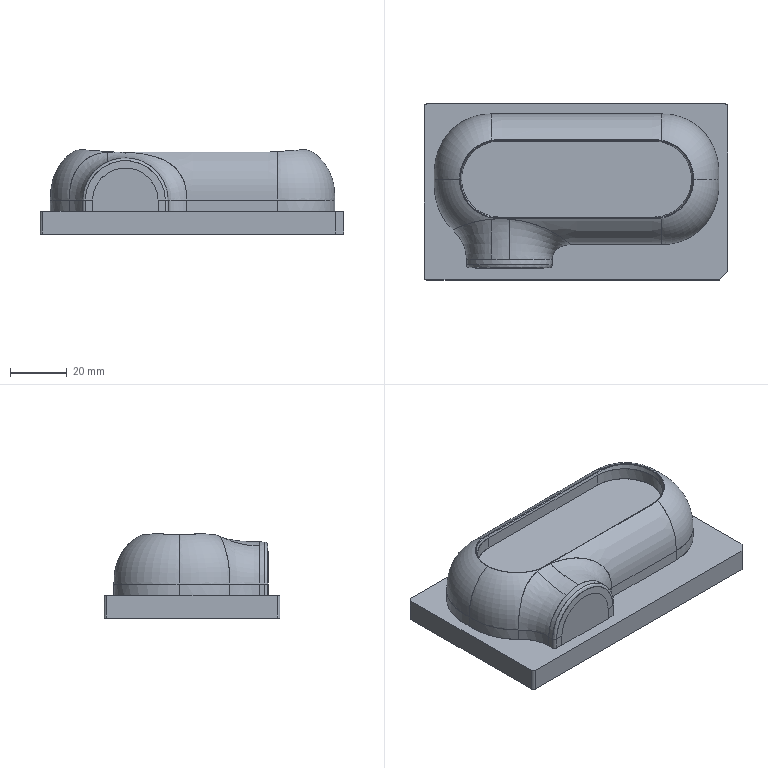NC program | PowerMill | posted by the shop | part box 107 x 62 x 29.663 mm
Lines 34277 to 35410 of 415021:
( TOOL ID   D10_1_1_1 )
( TOOL DIA. 10. TIP RAD 0 LENGTH 84.84 )
( Z = -6.359 )
T3 M6
T17
G91 G28 Z0
G0 G90 G54
M08
S8500 M3
X0 Y0 M8
G43 Z11.802 H3
X-19.327 Y8.267
Z-5.059
G1 Z-6.259 F360
X-25.057 Y8.319 Z-6.359
G3 X-28.917 Y4.509 I-.035 J-3.825 F600
X-25.087 Y.668 I3.825 J-.015
G1 X25.805 Y.724
G3 X25.833 Y7.858 I-.004 J3.567
G1 X-25.057 Y8.319
X-25.019 Y12.498
X-27.025 Y12.494
X-27.593 Y12.467
G3 X-28.444 Y12.348 I.713 J-8.214
G1 X-28.728 Y12.288
G3 X-29.42 Y12.093 I1.854 J-7.911
G1 X-29.863 Y11.932
G3 X-30.431 Y11.681 I3.427 J-8.517
X-30.999 Y11.374 I4.054 J-8.174
G1 X-31.282 Y11.197
X-31.615 Y10.968
X-31.884 Y10.763
X-32.134 Y10.557
X-32.304 Y10.406
X-32.503 Y10.218
X-32.701 Y10.017
X-32.869 Y9.835
X-33.074 Y9.598
X-33.323 Y9.281
X-33.524 Y8.999
X-33.707 Y8.718
X-33.837 Y8.502
X-34.025 Y8.156
X-34.163 Y7.875
X-34.287 Y7.593
X-34.404 Y7.3
X-34.499 Y7.031
X-34.587 Y6.75
X-34.663 Y6.47
X-34.73 Y6.187
G3 X-34.864 Y5.359 I8.12 J-1.736
G1 X-34.905 Y4.781
Y4.219
X-34.866 Y3.656
X-34.831 Y3.375
X-34.785 Y3.093
X-34.73 Y2.813
G3 X-34.404 Y1.7 I8.131 J1.778
G1 X-34.287 Y1.407
G3 X-34.025 Y.844 I8.475 J3.609
G1 X-33.837 Y.498
X-33.707 Y.282
X-33.524 Y.001
X-33.269 Y-.353
G3 X-32.863 Y-.843 I7.187 J5.55
G1 X-32.701 Y-1.017
X-32.503 Y-1.218
G3 X-31.566 Y-2.003 I5.801 J5.972
G1 X-31.282 Y-2.197
G3 X-30.037 Y-2.859 I4.373 J6.723
G1 X-29.863 Y-2.932
X-29.42 Y-3.093
G3 X-28.444 Y-3.348 I2.55 J7.756
G1 X-28.16 Y-3.398
X-27.593 Y-3.467
X-27.309 Y-3.485
X-27.025 Y-3.494
X-26.458 Y-3.498
X27.248 Y-3.496
X27.599 Y-3.49
X27.816 Y-3.482
X28.033 Y-3.467
X28.317 Y-3.438
X28.601 Y-3.398
X28.884 Y-3.348
G3 X29.86 Y-3.093 I-1.564 J7.957
G1 X30.303 Y-2.932
X30.589 Y-2.811
X30.871 Y-2.681
X31.164 Y-2.53
X31.439 Y-2.374
X31.722 Y-2.197
X32.055 Y-1.968
X32.314 Y-1.771
G3 X32.773 Y-1.379 I-5.391 J6.764
G1 X32.943 Y-1.218
X33.148 Y-1.011
X33.304 Y-.843
X33.514 Y-.598
X33.763 Y-.281
X33.964 Y.001
X34.147 Y.282
X34.277 Y.498
X34.465 Y.844
X34.603 Y1.125
X34.728 Y1.407
G3 X34.939 Y1.969 I-8.211 J3.408
G1 X35.026 Y2.249
X35.104 Y2.531
G3 X35.269 Y3.365 I-8.092 J2.037
G1 X35.306 Y3.656
X35.345 Y4.219
Y4.781
X35.306 Y5.344
X35.27 Y5.626
X35.226 Y5.906
G3 X34.947 Y7.007 I-8.097 J-1.467
G1 X34.844 Y7.3
G3 X34.603 Y7.875 I-8.957 J-3.416
G1 X34.465 Y8.156
X34.277 Y8.502
X34.147 Y8.718
X33.964 Y8.999
X33.763 Y9.281
G3 X33.141 Y10.017 I-6.537 J-4.887
G1 X32.943 Y10.218
X32.745 Y10.406
X32.532 Y10.591
X32.314 Y10.771
X32.055 Y10.968
G3 X31.439 Y11.374 I-5.546 J-7.74
G1 X31.164 Y11.53
X30.871 Y11.681
X30.589 Y11.811
X30.303 Y11.932
X30.02 Y12.035
X29.736 Y12.133
G3 X28.884 Y12.348 I-2.437 J-7.865
G1 X28.601 Y12.398
X28.317 Y12.437
X28.033 Y12.467
X27.465 Y12.494
X26.898 Y12.498
X-25.019
X-25.057 Y8.319
G0 Z11.802
X0 Y0
Z9.784
X64.2 Y6.547
Z-20.66
G1 Z-21.86 F360
X58.925 F600
X55.775 Y6.525
X55.776 Y2.383
G2 X55.632 Y-.364 I-30.159 J.203
G1 X55.555 Y-1.057
X55.471 Y-1.684
X55.374 Y-2.309
X55.263 Y-2.93
X55.144 Y-3.525
X55.011 Y-4.118
X54.897 Y-4.589
X54.767 Y-5.079
X54.63 Y-5.568
G2 X53.817 Y-7.944 I-26.15 J7.621
X52.595 Y-10.601 I-24.535 J9.675
G1 X52.226 Y-11.275
X51.836 Y-11.938
X51.516 Y-12.452
X51.249 Y-12.86
X50.861 Y-13.425
X50.457 Y-13.98
X50.035 Y-14.526
X49.535 Y-15.138
X49.502 Y-15.176
X53.081 Y-18.384
G2 X54.12 Y-18.799 I.444 J-.398
G1 X53.881 Y-27.29
G2 X53.366 Y-28.574 I-1.999 J.056
G1 X51.521 Y-30.619
G2 X50.862 Y-31.101 I-1.485 J1.34
G1 X50.317 Y-31.347
G2 X49.495 Y-31.526 I-.826 J1.822
G1 X1.462 Y-31.616
G2 X.743 Y-30.445 I-.002 J.805
G1 X1.061 Y-29.824
G2 X2.841 Y-28.735 I1.781 J-.91
G1 X30.248 Y-28.724
X31.57 Y-28.696
X31.976 Y-28.676
G3 X36.07 Y-28.182 I-1.584 J30.354
G1 X36.164 Y-28.165
G3 X44.345 Y-25.323 I-5.549 J29.178
G1 X44.396 Y-25.297
G3 X49.758 Y-21.686 I-13.363 J25.632
G1 X49.79 Y-21.659
G3 X52.598 Y-18.924 I-18.78 J22.085
G1 X53.081 Y-18.384
X49.502 Y-15.176
X49.087 Y-15.653
X48.676 Y-16.101
X48.195 Y-16.599
X47.702 Y-17.082
X47.198 Y-17.549
X46.68 Y-18.002
X46.148 Y-18.441
X45.725 Y-18.774
G2 X43.959 Y-20.01 I-14.692 J19.109
G1 X43.446 Y-20.328
G2 X42.088 Y-21.088 I-12.386 J20.529
G1 X41.605 Y-21.332
G2 X40.454 Y-21.859 I-9.151 J18.475
G1 X40.032 Y-22.037
X39.266 Y-22.336
G2 X38.278 Y-22.678 I-8.51 J23.
G1 X37.622 Y-22.879
X36.962 Y-23.063
X36.438 Y-23.195
X36.075 Y-23.281
X35.709 Y-23.36
X35.222 Y-23.458
G2 X31.391 Y-23.898 I-4.914 J25.859
X30.27 Y-23.921 I-1.135 J27.526
G1 X-1.78
X-1.965 Y-23.926
X-2.137 Y-23.941
G3 X-3.017 Y-24.934 I.121 J-.993
G1 Y-25.671
X-3.023 Y-25.924
X-3.039 Y-26.176
X-3.061 Y-26.419
X-3.094 Y-26.66
G2 X-3.218 Y-27.262 I-8.315 J1.397
G1 X-3.281 Y-27.492
G2 X-3.481 Y-28.065 I-8.097 J2.497
G1 X-3.573 Y-28.282
G2 X-3.836 Y-28.809 I-7.805 J3.582
G1 X-3.947 Y-28.999
X-4.093 Y-29.227
X-4.246 Y-29.449
G2 X-4.889 Y-30.203 I-5.42 J3.97
X-5.349 Y-30.622 I-6.037 J6.161
G1 X-5.545 Y-30.778
G2 X-6.043 Y-31.122 I-5.162 J6.942
G1 X-6.227 Y-31.233
X-6.463 Y-31.362
X-6.702 Y-31.482
X-6.901 Y-31.571
G2 X-7.473 Y-31.786 I-3.322 J7.975
G1 X-7.715 Y-31.859
G2 X-8.309 Y-31.995 I-2.225 J8.37
G1 X-8.522 Y-32.029
X-8.837 Y-32.066
X-9.107 Y-32.087
X-11.656 Y-32.221
X-11.939 Y-32.228
X-35.057
X-35.34 Y-32.221
X-37.889 Y-32.087
X-38.133 Y-32.068
X-38.377 Y-32.041
X-38.611 Y-32.008
X-38.842 Y-31.965
G2 X-39.42 Y-31.818 I1.79 J8.253
G1 X-39.64 Y-31.747
G2 X-40.187 Y-31.53 I2.845 J7.991
G1 X-40.394 Y-31.433
X-40.651 Y-31.297
X-40.903 Y-31.153
X-41.091 Y-31.033
X-41.322 Y-30.872
X-41.547 Y-30.703
X-41.717 Y-30.564
G2 X-42.143 Y-30.167 I5.425 J6.254
G1 X-42.309 Y-29.991
G2 X-42.714 Y-29.498 I6.378 J5.656
G1 X-42.862 Y-29.29
G2 X-43.182 Y-28.769 I7.242 J4.805
G1 X-43.215 Y-28.706
X-47.701 Y-30.518
G2 X-48.47 Y-31.618 I-.742 J-.3
G1 X-51.833 Y-31.505
G2 X-54.094 Y-29.172 I.078 J2.338
G1 X-54.114 Y-18.241
G2 X-53.079 Y-17.86 I.587 J.001
G1 X-50.382 Y-21.029
G2 X-48.836 Y-24.886 I-4.971 J-4.232
G1 X-48.719 Y-26.813
X-48.685 Y-27.113
G3 X-47.98 Y-29.827 I10.742 J1.341
G1 X-47.701 Y-30.518
X-43.215 Y-28.706
X-43.282 Y-28.581
X-43.396 Y-28.344
X-43.501 Y-28.103
X-43.579 Y-27.902
G2 X-43.764 Y-27.319 I8.157 J2.911
G1 X-43.825 Y-27.071
G2 X-43.929 Y-26.466 I8.479 J1.781
G1 X-43.953 Y-26.251
X-43.973 Y-25.936
X-43.979 Y-25.671
Y-23.789
X-43.986 Y-23.413
X-44.004 Y-23.085
X-44.025 Y-22.836
X-44.063 Y-22.526
X-44.111 Y-22.226
X-44.162 Y-21.966
X-44.227 Y-21.69
X-44.299 Y-21.424
X-44.428 Y-21.021
X-44.542 Y-20.719
X-44.699 Y-20.352
X-44.706 Y-20.337
G3 X-45.617 Y-18.826 I-7.564 J-3.53
G1 X-45.855 Y-18.525
X-46.096 Y-18.24
G3 X-46.943 Y-17.381 I-9.233 J-8.252
G1 X-47.569 Y-16.784
X-48.081 Y-16.264
X-48.581 Y-15.726
X-49.029 Y-15.217
X-49.211 Y-15.
X-49.7 Y-14.394
X-50.17 Y-13.774
X-50.525 Y-13.276
G2 X-51.562 Y-11.662 I20.702 J14.437
X-52.307 Y-10.31 I22.239 J13.135
G1 X-52.512 Y-9.901
G2 X-53.381 Y-7.933 I23.744 J11.664
G1 X-53.644 Y-7.241
X-53.885 Y-6.547
G2 X-54.709 Y-3.498 I26.377 J8.768
X-55.26 Y.433 I28.513 J5.997
X-55.335 Y2.365 I29.628 J2.131
G1 X-55.336 Y6.617
G2 X-55.192 Y9.364 I30.157 J-.203
G1 X-55.115 Y10.057
X-55.031 Y10.684
X-54.934 Y11.309
X-54.823 Y11.93
X-54.704 Y12.525
X-54.572 Y13.116
X-54.457 Y13.587
X-54.327 Y14.078
X-54.19 Y14.568
G2 X-53.499 Y16.629 I26.181 J-7.63
X-52.154 Y19.602 I24.703 J-9.383
G1 X-51.784 Y20.279
X-51.392 Y20.944
X-50.941 Y21.661
X-50.616 Y22.143
X-50.421 Y22.425
X-50.051 Y22.933
X-49.595 Y23.526
X-49.441 Y23.716
X-53.087 Y26.857
G2 X-54.117 Y27.253 I-.445 J.381
G1 X-54.064 Y29.217
G2 X-51.646 Y31.596 I2.444 J-.065
G1 X-49.856 Y31.614
G2 X-49.454 Y30.579 I.006 J-.593
G1 X-49.96 Y30.126
G3 X-51.935 Y28.171 I18.528 J-20.696
G1 X-52.35 Y27.711
X-53.087 Y26.857
X-49.441 Y23.716
X-49.094 Y24.139
X-48.646 Y24.653
X-48.236 Y25.101
X-47.755 Y25.599
X-47.262 Y26.082
X-46.757 Y26.549
X-46.239 Y27.002
X-45.708 Y27.442
X-45.284 Y27.774
G2 X-43.51 Y29.016 I14.7 J-19.123
G1 X-43.004 Y29.328
G2 X-41.648 Y30.088 I12.413 J-20.582
G1 X-41.165 Y30.332
X-40.79 Y30.513
X-40.41 Y30.687
X-39.863 Y30.925
X-39.194 Y31.196
X-38.878 Y31.316
G2 X-37.837 Y31.678 I8.482 J-22.752
G1 X-37.182 Y31.879
X-36.522 Y32.063
X-35.999 Y32.195
X-35.635 Y32.28
X-35.27 Y32.36
X-34.789 Y32.456
G2 X-33.086 Y32.723 I4.886 J-25.636
G1 X-32.611 Y32.777
G2 X-30.32 Y32.917 I2.762 J-26.423
G1 X-29.829 Y32.921
X30.338
X31.029 Y32.91
X31.716 Y32.882
X32.377 Y32.839
X33.039 Y32.778
X33.716 Y32.699
X34.39 Y32.602
X35.053 Y32.489
X35.711 Y32.36
G2 X37.528 Y31.907 I-5.288 J-25.073
G1 X38.213 Y31.698
G2 X41.011 Y30.614 I-7.55 J-23.643
G1 X41.544 Y30.362
X42.07 Y30.098
X42.475 Y29.883
G2 X43.354 Y29.383 I-11.366 J-21.016
G1 X43.841 Y29.085
X44.215 Y28.846
X44.789 Y28.458
G2 X46.655 Y27.023 I-14.02 J-20.16
G1 X49.898 Y30.579
G2 X50.316 Y31.617 I.399 J.443
G1 X51.707 Y31.573
G2 X54.099 Y29.128 I-.079 J-2.47
G1 X54.113 Y27.805
G2 X53.072 Y27.4 I-.597 J-.006
G1 X52.337 Y28.213
X51.455 Y29.13
X50.929 Y29.639
X49.898 Y30.579
X46.655 Y27.023
G2 X48.063 Y25.731 I-15.887 J-18.726
G1 X48.562 Y25.222
X48.987 Y24.763
G2 X49.878 Y23.723 I-17.653 J-16.022
X50.887 Y22.388 I-19.385 J-15.697
G1 X51.19 Y21.948
G2 X52.669 Y19.46 I-21.318 J-14.358
G1 X53.037 Y18.727
X53.369 Y18.012
G2 X53.788 Y17.018 I-24.088 J-10.741
G1 X54.029 Y16.391
X54.253 Y15.758
X54.422 Y15.248
X54.532 Y14.899
X54.636 Y14.549
G2 X54.92 Y13.494 I-27.366 J-7.941
G1 X55.043 Y12.982
X55.155 Y12.468
X55.251 Y11.995
G2 X55.452 Y10.811 I-27.501 J-5.296
G1 X55.54 Y10.178
G2 X55.771 Y6.96 I-29.288 J-3.724
G1 X55.775 Y6.525
X58.925 Y6.547
G0 Z9.784
Z10.802
X0 Y0
X40.365 Y-27.917
Z-20.63
G1 Z-21.83 F360
G3 X38.447 Y-22.232 I-.959 J2.843 F600
G2 X34.241 Y-23.251 I-7.89 J23.381
X30.213 Y-23.551 I-3.959 J25.943
G1 X-1.734
G3 X-3.074 Y-23.792 I-.062 J-3.512
X-3.268 Y-23.879 I.644 J-1.692
X-3.387 Y-24.074 I.101 J-.195
G1 Y-25.65
G2 X-9.032 Y-31.712 I-6.057 J-.018
G1 X-11.589 Y-31.847
G2 X-11.957 Y-31.858 I-.362 J5.715
G1 X-35.145 Y-31.857
X-35.329 Y-31.851
X-37.886 Y-31.717
G2 X-43.609 Y-25.649 I.333 J6.047
G1 Y-23.824
G3 X-43.8 Y-21.89 I-9.051 J.083
X-45.144 Y-18.848 I-8.09 J-1.757
X-46.481 Y-17.309 I-8.622 J-6.139
G2 X-47.43 Y-16.401 I23.417 J25.426
X-52.009 Y-10.08 I17.615 J17.578
X-54.463 Y-2.844 I24.033 J12.184
X-54.966 Y2.465 I28.77 J5.405
X-54.965 Y6.664 I735.857 J1.971
X-53.919 Y14.17 I28.79 J-.187
X-50.909 Y21.024 I25.297 J-7.021
X-43.766 Y28.408 I20.748 J-12.925
X-34.609 Y32.114 I13.602 J-20.443
X-29.848 Y32.551 I4.757 J-25.639
G1 X.365
X21.283
X30.213
G2 X38.454 Y31.23 I.112 J-25.653
X50.542 Y22.235 I-7.73 J-23.008
X54.254 Y14.535 I-21.245 J-14.987
X55.405 Y6.664 I-27.545 J-8.048
X55.406 Y2.464 I-614.971 J-2.231
X54.183 Y-5.774 I-28.696 J.052
X50.765 Y-12.916 I-24.901 J7.529
X43.77 Y-19.693 I-20.108 J13.758
X38.447 Y-22.232 I-13.212 J20.842
G3 X40.365 Y-27.917 I.959 J-2.843
G1 X40.258 Y-27.869
G3 X38.356 Y-22.179 I-.951 J2.845
G2 X34.229 Y-23.172 I-7.798 J23.326
X30.213 Y-23.471 I-3.947 J25.863
G1 X-1.734
G3 X-3.231 Y-23.771 I-.066 J-3.552
G1 X-3.304 Y-23.808
G3 X-3.467 Y-24.074 I.137 J-.267
G1 Y-25.649
G2 X-9.037 Y-31.632 I-5.977 J-.019
G1 X-11.592 Y-31.767
G2 X-11.957 Y-31.778 I-.358 J5.622
G1 X-34.96
G2 X-35.325 Y-31.771 I-.068 J5.794
G1 X-37.88 Y-31.637
G2 X-43.529 Y-25.649 I.328 J5.968
G1 Y-23.824
G3 X-43.722 Y-21.872 I-9.13 J.082
X-45.079 Y-18.802 I-8.168 J-1.774
X-46.426 Y-17.252 I-8.688 J-6.185
G2 X-47.373 Y-16.345 I23.386 J25.393
X-51.937 Y-10.045 I17.558 J17.522
X-54.384 Y-2.83 I23.961 J12.148
X-54.886 Y2.465 I28.691 J5.391
X-54.885 Y6.663 I737.797 J1.972
X-53.627 Y14.878 I28.591 J-.175
X-50.112 Y22.083 I24.74 J-7.612
X-38.072 Y31.126 I19.831 J-13.867
X-29.848 Y32.471 I8.181 J-24.199
G1 X.365
X21.283
X30.213
G2 X38.793 Y31.028 I.117 J-25.53
X50.477 Y22.189 I-8.067 J-22.805
X54.177 Y14.513 I-21.179 J-14.941
X55.325 Y6.663 I-27.468 J-8.026
X55.326 Y2.465 I-614.241 J-2.231
X54.106 Y-5.751 I-28.616 J.051
X50.699 Y-12.87 I-24.825 J7.505
X43.727 Y-19.625 I-20.042 J13.712
X38.356 Y-22.179 I-13.169 J20.772
G3 X40.258 Y-27.869 I.951 J-2.845
G0 Z3.857
G1 X7.364 Y2.132 F10000
G0 Z-5.159
G1 Z-6.359 F360
G3 X7.364 Y-3.868 I0 J-3. F600
G1 X27.267
G3 X30.13 Y-3.392 I.052 J8.542
X32.889 Y-1.774 I-2.808 J7.949
X35.677 Y5.351 I-5.54 J6.276
X31.785 Y11.596 I-8.323 J-.852
X27.949 Y12.845 I-4.432 J-7.097
X27.267 Y12.867 I-.714 J-11.242
G1 X21.283
X.374
X-26.637
G3 X-28.201 Y12.766 I-.181 J-9.346
X-32.217 Y10.971 I1.295 J-8.286
X-32.575 Y10.659 I8.438 J-10.045
G1 X-32.898 Y10.347
X-33.187 Y10.035
G3 X-33.56 Y-.582 I6.274 J-5.535
X-27.265 Y-3.858 I6.65 J5.091
X-26.637 Y-3.867 I.566 J18.02
G1 X7.364 Y-3.868
G3 X7.364 Y2.132 I0 J3.
G0 Z3.857
G1 X7.5 Y2.052 F10000
G0 Z-5.159
G1 Z-6.359 F360
G3 X7.5 Y-3.948 I0 J-3. F600
G1 X27.268
G3 X30.157 Y-3.468 I.051 J8.622
X32.942 Y-1.834 I-2.835 J8.025
X35.757 Y5.359 I-5.593 J6.336
X31.827 Y11.664 I-8.402 J-.86
X27.954 Y12.925 I-4.474 J-7.165
X27.268 Y12.947 I-.715 J-11.181
G1 X21.283
X.374
X-26.637
G3 X-28.214 Y12.845 I-.181 J-9.424
X-32.268 Y11.033 I1.307 J-8.365
X-32.63 Y10.718 I8.534 J-10.16
G1 X-32.955 Y10.403
X-33.247 Y10.088
G3 X-33.624 Y-.63 I6.334 J-5.588
X-27.268 Y-3.938 I6.714 J5.139
X-26.637 Y-3.947 I.569 J18.109
G1 X7.5 Y-3.948
G3 X7.5 Y2.052 I0 J3.
G0 Z10.802
X0 Y0
Z9.784
X58.482 Y-37.273
Z-28.56
G1 Z-29.76 F360
G3 X54.947 Y-33.738 I-1.768 J1.768 F600
G1 X54.326 Y-34.358
Y-34.359
X54.325
X53.959 Y-34.72
X53.957 Y-34.722
X53.955 Y-34.724
X53.639 Y-34.994
X53.636 Y-34.996
X53.634 Y-34.998
X53.317 Y-35.227
X53.316 Y-35.228
X53.314 Y-35.23
X53.177 Y-35.318
X53.176
X53.174 Y-35.319
X52.995 Y-35.425
X52.993 Y-35.426
X52.991 Y-35.427
X52.675 Y-35.591
X52.673 Y-35.592
X52.672
X52.57 Y-35.639
X52.569 Y-35.64
X52.568
X52.353 Y-35.73
X52.351 Y-35.731
X52.349 Y-35.732
X52.033 Y-35.843
X52.03 Y-35.844
X52.028 Y-35.845
X51.711 Y-35.933
X51.71 Y-35.934
X51.708
X51.596 Y-35.96
X51.594 Y-35.961
X51.593
X51.389 Y-36.002
X51.387
X51.385
X51.069 Y-36.048
X51.066
X51.064 Y-36.049
X50.748 Y-36.074
X50.745
X50.743
X50.427 Y-36.08
X50.426
X50.425
X-52.322
X-52.323
X-52.639 Y-36.078
X-52.64
X-52.642
X-52.958 Y-36.063
X-52.96
X-52.963 Y-36.062
X-53.279 Y-36.03
X-53.281
X-53.283 Y-36.029
X-53.599 Y-35.98
X-53.601 Y-35.979
X-53.603
X-53.919 Y-35.912
X-53.922 Y-35.911
X-53.924
X-54.24 Y-35.826
X-54.242 Y-35.825
X-54.244 Y-35.824
X-54.56 Y-35.72
X-54.562 Y-35.719
X-54.564 Y-35.718
X-54.88 Y-35.595
X-54.883 Y-35.594
X-54.885 Y-35.593
X-55.201 Y-35.447
X-55.203 Y-35.446
X-55.205 Y-35.445
X-55.521 Y-35.276
X-55.523 Y-35.275
X-55.525 Y-35.274
X-55.842 Y-35.079
X-55.843 Y-35.078
X-55.844 Y-35.077
X-55.959 Y-35.
X-55.96
X-55.961 Y-34.999
X-56.163 Y-34.853
X-56.164 Y-34.852
X-56.166 Y-34.851
X-56.38 Y-34.681
X-56.381 Y-34.68
X-56.382 Y-34.679
X-56.484 Y-34.593
X-56.485 Y-34.592
X-56.486 Y-34.591
X-56.737 Y-34.361
X-56.738 Y-34.36
X-56.739 Y-34.359
X-56.804 Y-34.294
X-56.805 Y-34.293
X-56.806 Y-34.292
X-57.043 Y-34.04
X-57.044 Y-34.039
X-57.045 Y-34.038
X-57.125 Y-33.946
X-57.126 Y-33.945
Y-33.944
X-57.309 Y-33.72
X-57.31 Y-33.719
X-57.311 Y-33.717
X-57.445 Y-33.538
X-57.446 Y-33.537
Y-33.535
X-57.54 Y-33.399
X-57.541 Y-33.397
X-57.542 Y-33.396
X-57.742 Y-33.08
X-57.743 Y-33.078
X-57.745 Y-33.076
X-57.918 Y-32.759
X-57.919 Y-32.757
X-57.92 Y-32.755
X-58.069 Y-32.439
X-58.07 Y-32.437
X-58.071 Y-32.435
X-58.199 Y-32.119
X-58.2 Y-32.117
Y-32.115
X-58.308 Y-31.798
X-58.309 Y-31.796
Y-31.794
X-58.397 Y-31.478
X-58.398 Y-31.476
X-58.399 Y-31.474
X-58.469 Y-31.158
Y-31.156
Y-31.153
X-58.522 Y-30.837
Y-30.835
X-58.523 Y-30.833
X-58.558 Y-30.517
Y-30.515
Y-30.513
X-58.576 Y-30.196
Y-30.195
Y-30.193
X-58.58 Y-29.877
Y-29.876
Y29.876
Y29.877
X-58.576 Y30.193
Y30.195
Y30.196
X-58.558 Y30.513
Y30.515
Y30.517
X-58.523 Y30.833
X-58.522 Y30.835
Y30.837
X-58.47 Y31.153
X-58.469 Y31.155
Y31.157
X-58.407 Y31.44
Y31.442
X-58.406 Y31.444
X-58.309 Y31.794
Y31.796
X-58.308 Y31.799
X-58.2 Y32.115
X-58.199 Y32.117
X-58.198 Y32.118
X-58.087 Y32.398
X-58.086 Y32.4
X-58.085 Y32.402
X-57.919 Y32.755
X-57.918 Y32.757
X-57.917 Y32.759
X-57.767 Y33.037
X-57.766 Y33.039
X-57.764 Y33.042
X-57.543 Y33.396
X-57.542 Y33.397
X-57.541 Y33.399
X-57.446 Y33.536
X-57.445 Y33.537
Y33.538
X-57.311 Y33.717
X-57.31 Y33.719
X-57.309 Y33.72
X-57.126 Y33.945
Y33.946
X-57.125 Y33.947
X-57.045 Y34.038
X-57.044 Y34.039
X-57.043 Y34.04
X-56.806 Y34.292
X-56.805 Y34.293
X-56.804 Y34.294
X-56.739 Y34.359
X-56.738 Y34.36
X-56.737 Y34.361
X-56.486 Y34.591
X-56.485 Y34.592
X-56.484 Y34.593
X-56.382 Y34.679
X-56.381 Y34.68
X-56.38 Y34.681
X-56.166 Y34.851
X-56.164 Y34.852
X-56.163 Y34.853
X-55.96 Y34.999
X-55.959 Y35.
X-55.958 Y35.001
X-55.844 Y35.077
X-55.843 Y35.078
X-55.842
X-55.526 Y35.274
X-55.523 Y35.275
X-55.521 Y35.276
X-55.205 Y35.445
X-55.203 Y35.446
X-55.201 Y35.447
X-54.885 Y35.593
X-54.883 Y35.594
X-54.881
X-54.564 Y35.719
X-54.562 Y35.72
X-54.56
X-54.244 Y35.824
X-54.242 Y35.825
X-54.24 Y35.826
X-53.924 Y35.911
X-53.922
X-53.92 Y35.912
X-53.698 Y35.961
X-53.696
X-53.694
X-53.284 Y36.029
X-53.281 Y36.03
X-53.279
X-52.962 Y36.062
X-52.96
X-52.958
X-52.642 Y36.078
X-52.64
X-52.639
X-52.323 Y36.08
X-52.322
X0
X52.322
X52.323
X52.639 Y36.078
X52.64
X52.642
X52.958 Y36.063
X52.96
X52.963 Y36.062
X53.279 Y36.03
X53.281
X53.283 Y36.029
X53.599 Y35.98
X53.601 Y35.979
X53.603
X53.919 Y35.912
X53.922 Y35.911
X53.924
X54.24 Y35.826
X54.242 Y35.825
X54.244 Y35.824
X54.56 Y35.72
X54.562 Y35.719
X54.564 Y35.718
X54.88 Y35.595
X54.883 Y35.594
X54.885 Y35.593
X55.201 Y35.447
X55.203 Y35.446
X55.205 Y35.445
X55.521 Y35.276
X55.523 Y35.275
X55.525 Y35.274
X55.842 Y35.079
X55.843 Y35.078
X55.844 Y35.077
X55.959 Y35.
X55.96
X55.961 Y34.999
X56.163 Y34.853
X56.164 Y34.852
X56.166 Y34.851
X56.38 Y34.681
X56.381 Y34.68
X56.382 Y34.679
X56.484 Y34.593
X56.485 Y34.592
X56.486 Y34.591
X56.737 Y34.361
X56.738 Y34.36
X56.739 Y34.359
X56.804 Y34.294
X56.805 Y34.293
X56.806 Y34.292
X57.043 Y34.04
X57.044 Y34.039
X57.045 Y34.038
X57.125 Y33.946
X57.126 Y33.945
Y33.944
X57.309 Y33.72
X57.31 Y33.719
X57.311 Y33.717
X57.445 Y33.538
X57.446 Y33.537
Y33.535
X57.54 Y33.399
X57.541 Y33.397
X57.542 Y33.396
X57.742 Y33.08
X57.743 Y33.078
X57.745 Y33.076
X57.918 Y32.759
X57.919 Y32.757
X57.92 Y32.755
X58.069 Y32.439
X58.07 Y32.437
X58.071 Y32.435
X58.199 Y32.119
X58.2 Y32.117
Y32.115
X58.308 Y31.798
X58.309 Y31.796
Y31.794
X58.397 Y31.478
X58.398 Y31.476
X58.399 Y31.474
X58.469 Y31.158
Y31.156
Y31.153
X58.522 Y30.837
Y30.835
X58.523 Y30.833
X58.558 Y30.517
Y30.515
Y30.513
X58.576 Y30.196
Y30.195
Y30.193
X58.58 Y29.877
Y29.876
Y-27.979
Y-27.98
Y-27.981
X58.571 Y-28.297
Y-28.3
Y-28.302
X58.542 Y-28.618
Y-28.621
Y-28.623
X58.492 Y-28.94
Y-28.942
X58.491 Y-28.945
X58.421 Y-29.261
X58.42 Y-29.263
Y-29.266
X58.327 Y-29.582
Y-29.585
X58.326 Y-29.587
X58.21 Y-29.903
X58.209 Y-29.906
X58.208 Y-29.908
X58.086 Y-30.185
X58.085 Y-30.188
X58.083 Y-30.19
X57.896 Y-30.545
X57.895 Y-30.548
X57.894 Y-30.55
X57.765 Y-30.76
X57.764 Y-30.761
X57.763 Y-30.763
X57.693 Y-30.869
X57.691 Y-30.87
X57.69 Y-30.872
X57.455 Y-31.188
X57.453 Y-31.191
X57.451 Y-31.193
X57.173 Y-31.509
X57.172 Y-31.511
X57.17 Y-31.512
X57.122 Y-31.562
X57.121 Y-31.563
X54.947 Y-33.738
G3 X58.482 Y-37.273 I1.768 J-1.768
G1 X58.431 Y-37.211
G3 X54.895 Y-33.676 I-1.768 J1.768
G1 X54.269 Y-34.302
X53.903 Y-34.663
X53.587 Y-34.933
X53.271 Y-35.162
X53.134 Y-35.25
X52.954 Y-35.356
X52.638 Y-35.52
X52.537 Y-35.566
X52.322 Y-35.656
X52.006 Y-35.768
X51.69 Y-35.856
X51.577 Y-35.883
X51.374 Y-35.923
X51.058 Y-35.969
X50.741 Y-35.994
X50.425 Y-36.
X-52.322
X-52.638 Y-35.998
X-52.954 Y-35.983
X-53.271 Y-35.95
X-53.587 Y-35.901
X-53.903 Y-35.834
X-54.219 Y-35.748
X-54.535 Y-35.644
X-54.851 Y-35.52
X-55.167 Y-35.374
X-55.484 Y-35.206
X-55.8 Y-35.011
X-55.914 Y-34.934
X-56.116 Y-34.788
X-56.331 Y-34.618
X-56.432 Y-34.532
X-56.683 Y-34.302
X-56.748 Y-34.237
X-56.985 Y-33.986
X-57.064 Y-33.894
X-57.247 Y-33.67
X-57.38 Y-33.49
X-57.475 Y-33.353
X-57.674 Y-33.037
X-57.847 Y-32.721
X-57.997 Y-32.405
X-58.125 Y-32.089
X-58.232 Y-31.773
X-58.32 Y-31.456
X-58.39 Y-31.14
X-58.443 Y-30.824
X-58.478 Y-30.508
X-58.496 Y-30.192
X-58.5 Y-29.876
Y29.876
X-58.496 Y30.192
X-58.478 Y30.508
X-58.443 Y30.824
X-58.391 Y31.14
X-58.329 Y31.423
X-58.232 Y31.773
X-58.124 Y32.089
X-58.013 Y32.368
X-57.847 Y32.721
X-57.697 Y32.999
X-57.475 Y33.353
X-57.38 Y33.49
X-57.247 Y33.67
X-57.064 Y33.894
X-56.985 Y33.986
X-56.748 Y34.237
X-56.682 Y34.302
X-56.432 Y34.532
X-56.33 Y34.618
X-56.116 Y34.788
X-55.913 Y34.934
X-55.8 Y35.01
X-55.484 Y35.206
X-55.167 Y35.374
X-54.851 Y35.52
X-54.535 Y35.644
X-54.219 Y35.748
X-53.903 Y35.834
X-53.681 Y35.883
X-53.271 Y35.95
X-52.954 Y35.982
X-52.638 Y35.998
X-52.322 Y36.
X0
X52.322
X52.638 Y35.998
X52.954 Y35.983
X53.271 Y35.95
X53.587 Y35.901
X53.903 Y35.834
X54.219 Y35.748
X54.535 Y35.644
X54.851 Y35.52
X55.167 Y35.374
X55.484 Y35.206
X55.8 Y35.011
X55.914 Y34.934
X56.116 Y34.788
X56.331 Y34.618
X56.432 Y34.532
X56.683 Y34.302
X56.748 Y34.237
X56.985 Y33.986
X57.064 Y33.894
X57.247 Y33.67
X57.38 Y33.49
X57.475 Y33.353
X57.674 Y33.037
X57.847 Y32.721
X57.997 Y32.405
X58.125 Y32.089
X58.232 Y31.773
X58.32 Y31.456
X58.39 Y31.14
X58.443 Y30.824
X58.478 Y30.508
X58.496 Y30.192
X58.5 Y29.876
Y-27.979
X58.491 Y-28.295
X58.463 Y-28.611
X58.413 Y-28.927
X58.343 Y-29.243
X58.251 Y-29.56
X58.135 Y-29.876
X58.013 Y-30.153
X57.825 Y-30.508
X57.697 Y-30.718
X57.626 Y-30.824
X57.391 Y-31.14
X57.113 Y-31.456
X57.064 Y-31.507
X54.895 Y-33.676
G3 X58.431 Y-37.211 I1.768 J-1.768
G0 Z9.784
Z10.802
X0 Y0
M9
M5
M01